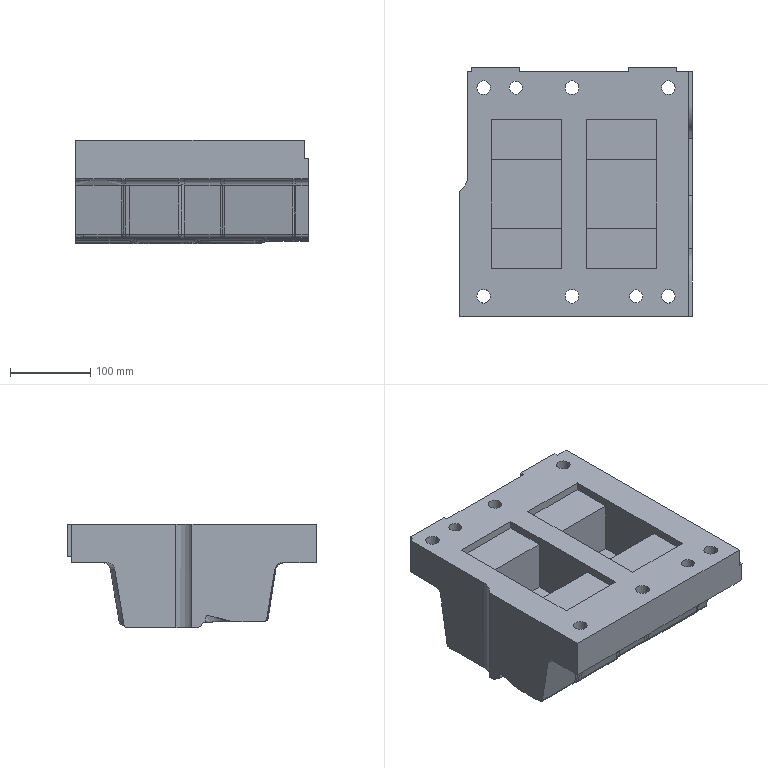Part | NX | features solid 2 | 1 solid | 227 faces | box 290 x 310 x 129.453 mm | volume 6904200 mm3 | spline 95 | plane 69 | cylinder 62 | sphere 1 | commonest cylinder face diameters 12 x16 8 x9 10 x8 20 x7 17 x6 26 x6